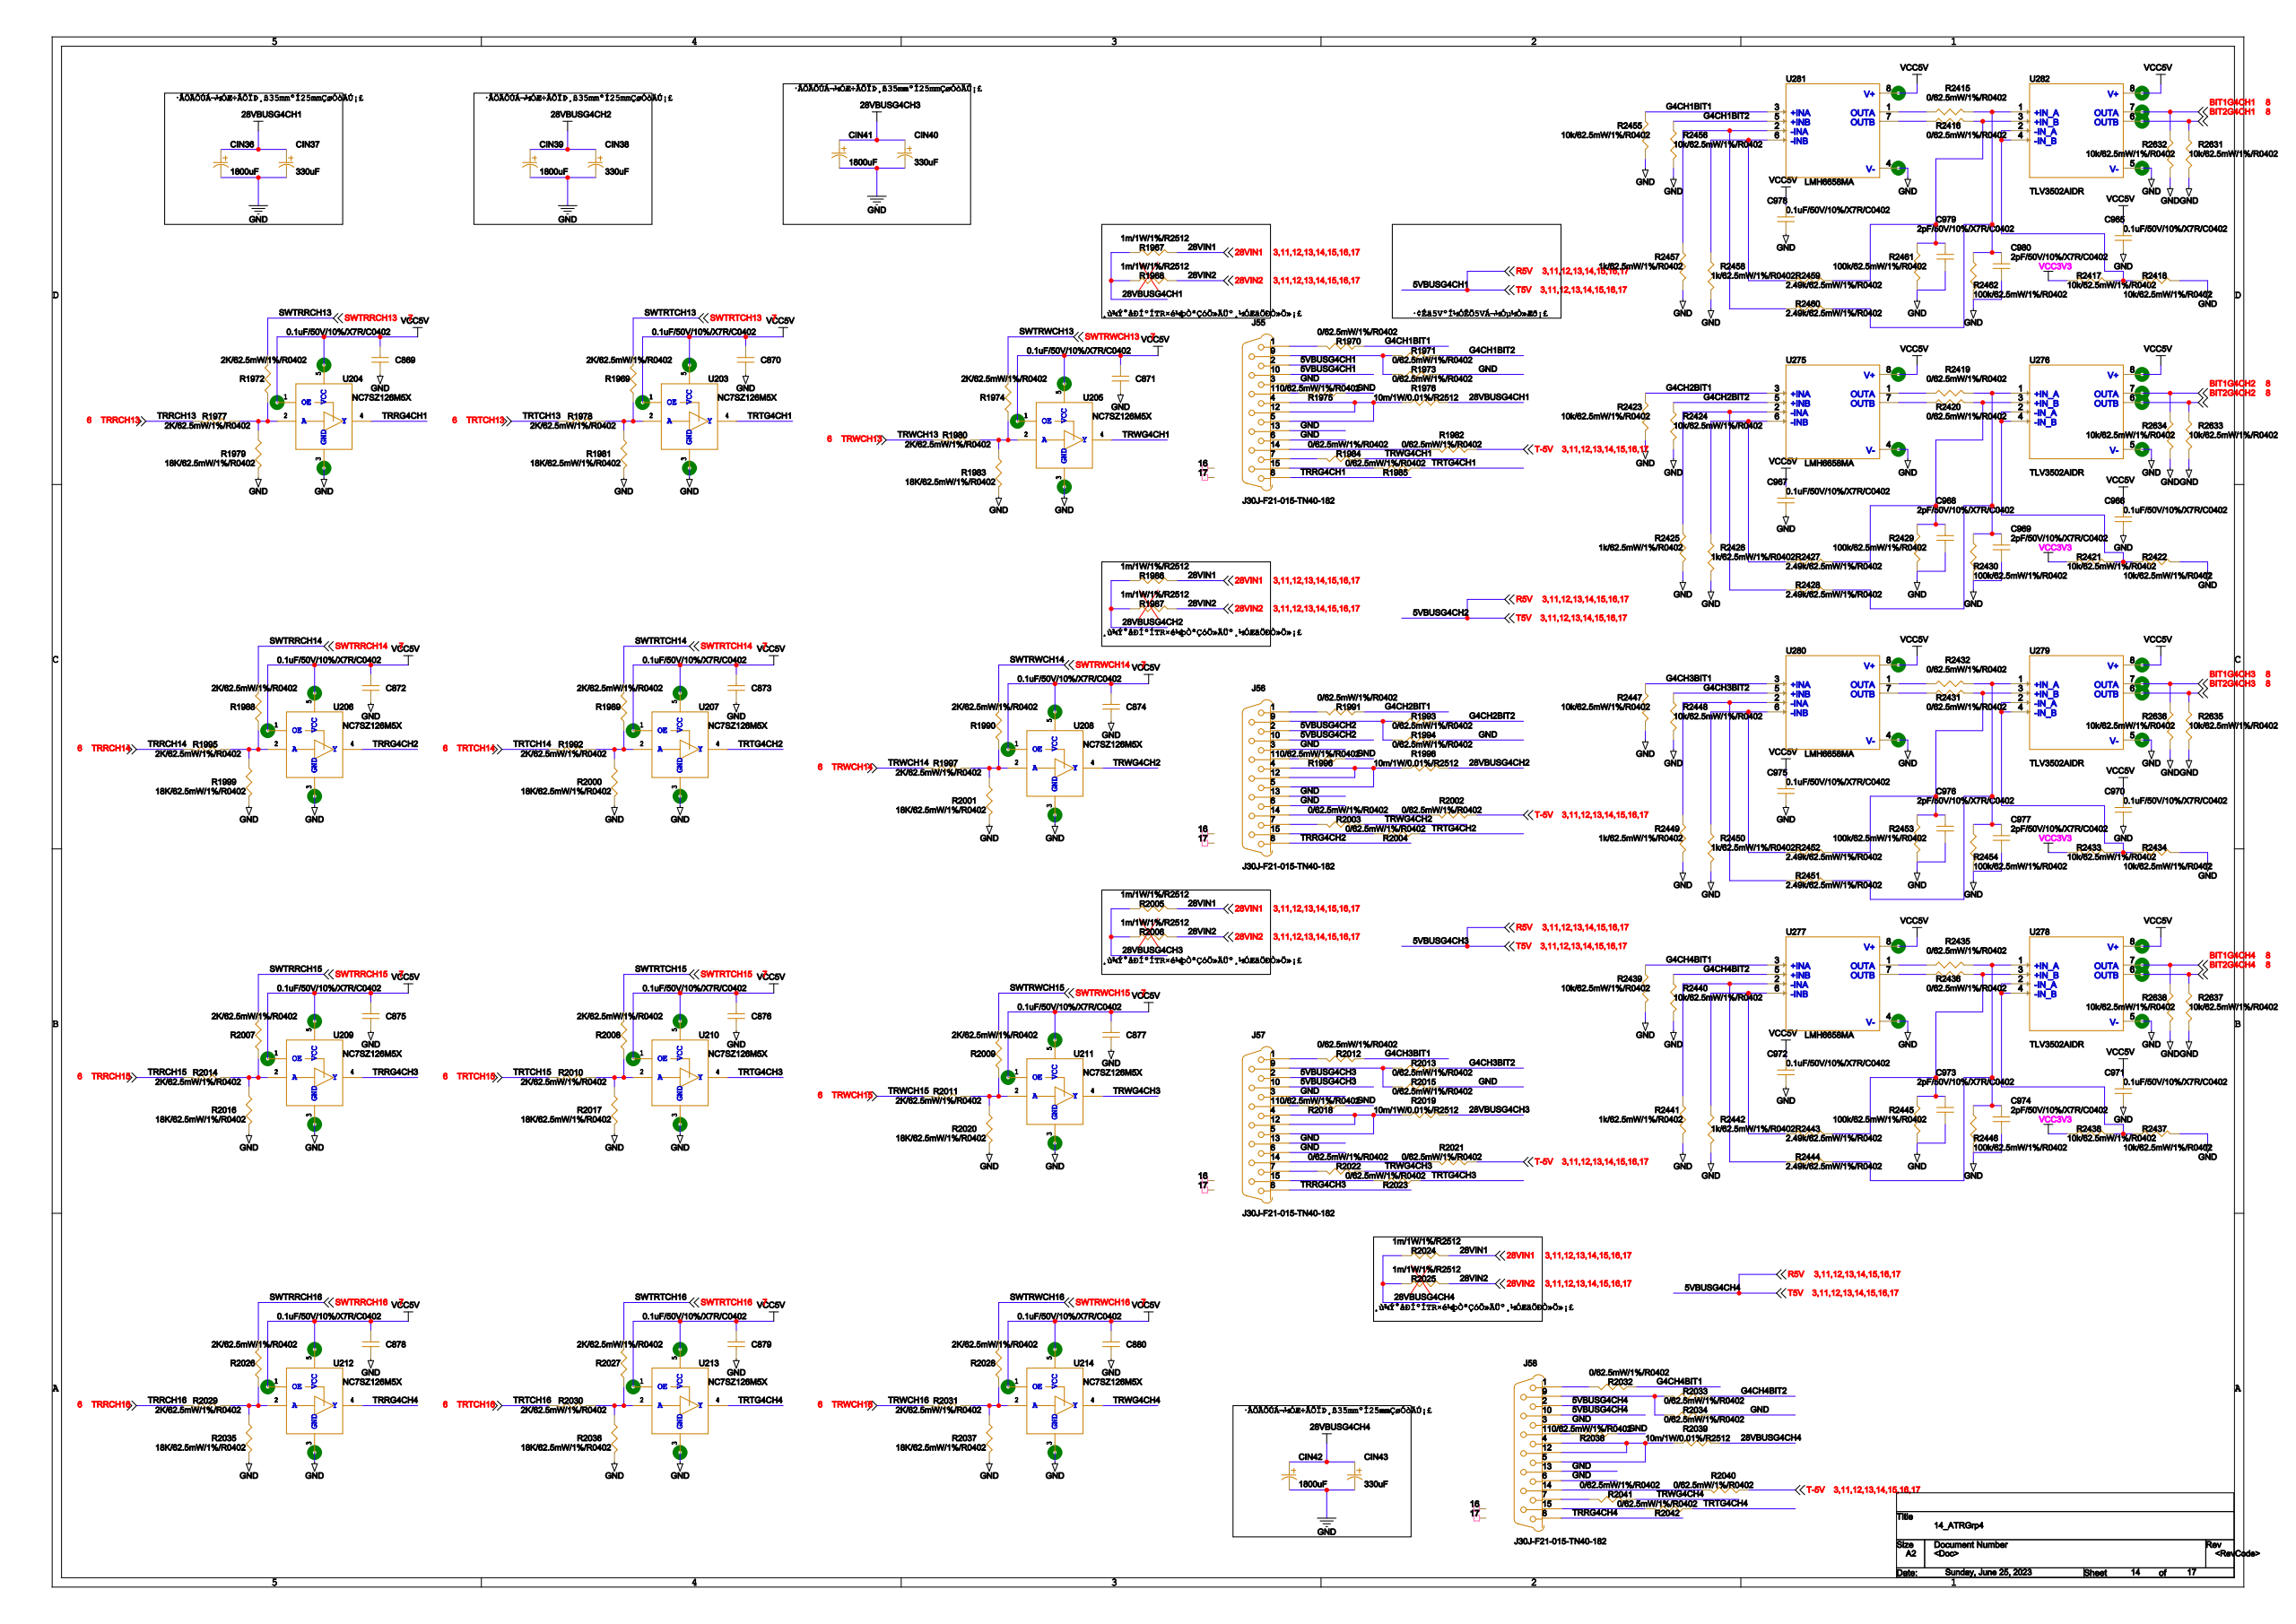Circuit board | Cadence Allegro | 2002 parts | 1538 nets | one sheet of the schematic
Parts on this sheet (reference | value | footprint):
C869 | 0.1uF/50V/10%/X7R/C0402 | 0402
C870 | 0.1uF/50V/10%/X7R/C0402 | 0402
C871 | 0.1uF/50V/10%/X7R/C0402 | 0402
C872 | 0.1uF/50V/10%/X7R/C0402 | 0402
C873 | 0.1uF/50V/10%/X7R/C0402 | 0402
C874 | 0.1uF/50V/10%/X7R/C0402 | 0402
C875 | 0.1uF/50V/10%/X7R/C0402 | 0402
C876 | 0.1uF/50V/10%/X7R/C0402 | 0402
C877 | 0.1uF/50V/10%/X7R/C0402 | 0402
C878 | 0.1uF/50V/10%/X7R/C0402 | 0402
C879 | 0.1uF/50V/10%/X7R/C0402 | 0402
C880 | 0.1uF/50V/10%/X7R/C0402 | 0402
C965 | 0.1uF/50V/10%/X7R/C0402 | 0402
C966 | 0.1uF/50V/10%/X7R/C0402 | 0402
C968 | 2pF/50V/10%/X7R/C0402 | 0402
C969 | 2pF/50V/10%/X7R/C0402 | 0402
C970 | 0.1uF/50V/10%/X7R/C0402 | 0402
C971 | 0.1uF/50V/10%/X7R/C0402 | 0402
C973 | 2pF/50V/10%/X7R/C0402 | 0402
C974 | 2pF/50V/10%/X7R/C0402 | 0402
C976 | 2pF/50V/10%/X7R/C0402 | 0402
C977 | 2pF/50V/10%/X7R/C0402 | 0402
C979 | 2pF/50V/10%/X7R/C0402 | 0402
C980 | 2pF/50V/10%/X7R/C0402 | 0402
CIN36 | ECF1HM182M27OTPO | AP-SMD_BD18-L27-W6_6-LS7_21
CIN37 | ECF1JM331G20OTPO | AP-SMD_BD10-L20-W6_6-LS7_21
CIN38 | ECF1JM331G20OTPO | AP-SMD_BD10-L20-W6_6-LS7_21
CIN39 | ECF1HM182M27OTPO | AP-SMD_BD18-L27-W6_6-LS7_21
CIN40 | ECF1JM331G20OTPO | AP-SMD_BD10-L20-W6_6-LS7_21
CIN41 | ECF1HM182M27OTPO | AP-SMD_BD18-L27-W6_6-LS7_21
CIN42 | ECF1HM182M27OTPO | AP-SMD_BD18-L27-W6_6-LS7_21
CIN43 | ECF1JM331G20OTPO | AP-SMD_BD10-L20-W6_6-LS7_21
J55 | J30J-F21-015-TN40-182 | J30J-F21-015-TN40-182
J56 | J30J-F21-015-TN40-182 | J30J-F21-015-TN40-182
J57 | J30J-F21-015-TN40-182 | J30J-F21-015-TN40-182
J58 | J30J-F21-015-TN40-182 | J30J-F21-015-TN40-182
R1967 | 1m/1W/1%/R2512 | 2512
R1968 | 1m/1W/1%/R2512 | 2512
R1969 | 2K/62.5mW/1%/R0402 | 0402
R1970 | 0/62.5mW/1%/R0402 | 0402
R1971 | 0/62.5mW/1%/R0402 | 0402
R1972 | 2K/62.5mW/1%/R0402 | 0402
R1973 | 0/62.5mW/1%/R0402 | 0402
R1974 | 2K/62.5mW/1%/R0402 | 0402
R1975 | 0/62.5mW/1%/R0402 | 0402
R1976 | 10m/1W/0.01%/R2512 | 2512
R1977 | 2K/62.5mW/1%/R0402 | 0402
R1978 | 2K/62.5mW/1%/R0402 | 0402
R1979 | 18K/62.5mW/1%/R0402 | 0402
R1980 | 2K/62.5mW/1%/R0402 | 0402
R1981 | 18K/62.5mW/1%/R0402 | 0402
R1982 | 0/62.5mW/1%/R0402 | 0402
R1983 | 18K/62.5mW/1%/R0402 | 0402
R1984 | 0/62.5mW/1%/R0402 | 0402
R1985 | 0/62.5mW/1%/R0402 | 0402
R1986 | 1m/1W/1%/R2512 | 2512
R1987 | 1m/1W/1%/R2512 | 2512
R1988 | 2K/62.5mW/1%/R0402 | 0402
R1989 | 2K/62.5mW/1%/R0402 | 0402
R1990 | 2K/62.5mW/1%/R0402 | 0402
R1991 | 0/62.5mW/1%/R0402 | 0402
R1992 | 2K/62.5mW/1%/R0402 | 0402
R1993 | 0/62.5mW/1%/R0402 | 0402
R1994 | 0/62.5mW/1%/R0402 | 0402
R1995 | 2K/62.5mW/1%/R0402 | 0402
R1996 | 0/62.5mW/1%/R0402 | 0402
R1997 | 2K/62.5mW/1%/R0402 | 0402
R1998 | 10m/1W/0.01%/R2512 | 2512
R1999 | 18K/62.5mW/1%/R0402 | 0402
R2000 | 18K/62.5mW/1%/R0402 | 0402
R2001 | 18K/62.5mW/1%/R0402 | 0402
R2002 | 0/62.5mW/1%/R0402 | 0402
R2003 | 0/62.5mW/1%/R0402 | 0402
R2004 | 0/62.5mW/1%/R0402 | 0402
R2005 | 1m/1W/1%/R2512 | 2512
R2006 | 1m/1W/1%/R2512 | 2512
R2007 | 2K/62.5mW/1%/R0402 | 0402
R2008 | 2K/62.5mW/1%/R0402 | 0402
R2009 | 2K/62.5mW/1%/R0402 | 0402
R2010 | 2K/62.5mW/1%/R0402 | 0402
R2011 | 2K/62.5mW/1%/R0402 | 0402
R2012 | 0/62.5mW/1%/R0402 | 0402
R2013 | 0/62.5mW/1%/R0402 | 0402
R2014 | 2K/62.5mW/1%/R0402 | 0402
R2015 | 0/62.5mW/1%/R0402 | 0402
R2016 | 18K/62.5mW/1%/R0402 | 0402
R2017 | 18K/62.5mW/1%/R0402 | 0402
R2018 | 0/62.5mW/1%/R0402 | 0402
R2019 | 10m/1W/0.01%/R2512 | 2512
R2020 | 18K/62.5mW/1%/R0402 | 0402
R2021 | 0/62.5mW/1%/R0402 | 0402
R2022 | 0/62.5mW/1%/R0402 | 0402
R2023 | 0/62.5mW/1%/R0402 | 0402
R2024 | 1m/1W/1%/R2512 | 2512
R2025 | 1m/1W/1%/R2512 | 2512
R2026 | 2K/62.5mW/1%/R0402 | 0402
R2027 | 2K/62.5mW/1%/R0402 | 0402
R2028 | 2K/62.5mW/1%/R0402 | 0402
R2029 | 2K/62.5mW/1%/R0402 | 0402
R2030 | 2K/62.5mW/1%/R0402 | 0402
R2031 | 2K/62.5mW/1%/R0402 | 0402
R2032 | 0/62.5mW/1%/R0402 | 0402
R2033 | 0/62.5mW/1%/R0402 | 0402
R2034 | 0/62.5mW/1%/R0402 | 0402
R2035 | 18K/62.5mW/1%/R0402 | 0402
R2036 | 18K/62.5mW/1%/R0402 | 0402
R2037 | 18K/62.5mW/1%/R0402 | 0402
R2038 | 0/62.5mW/1%/R0402 | 0402
R2039 | 10m/1W/0.01%/R2512 | 2512
R2040 | 0/62.5mW/1%/R0402 | 0402
R2041 | 0/62.5mW/1%/R0402 | 0402
R2042 | 0/62.5mW/1%/R0402 | 0402
R2415 | 0/62.5mW/1%/R0402 | 0402
R2416 | 0/62.5mW/1%/R0402 | 0402
R2417 | 10k/62.5mW/1%/R0402 | 0402
R2418 | 10k/62.5mW/1%/R0402 | 0402
R2419 | 0/62.5mW/1%/R0402 | 0402
R2420 | 0/62.5mW/1%/R0402 | 0402
R2421 | 10k/62.5mW/1%/R0402 | 0402
R2422 | 10k/62.5mW/1%/R0402 | 0402
R2423 | 10k/62.5mW/1%/R0402 | 0402
R2424 | 10k/62.5mW/1%/R0402 | 0402
R2425 | 1K/62.5mW/1%/R0402 | 0402
R2426 | 1K/62.5mW/1%/R0402 | 0402
R2428 | 2.49k/62.5mW/1%/R0402 | 0402
R2429 | 100k/62.5mW/1%/R0402 | 0402
R2430 | 100k/62.5mW/1%/R0402 | 0402
R2431 | 0/62.5mW/1%/R0402 | 0402
R2432 | 0/62.5mW/1%/R0402 | 0402
R2433 | 10k/62.5mW/1%/R0402 | 0402
R2434 | 10k/62.5mW/1%/R0402 | 0402
R2435 | 0/62.5mW/1%/R0402 | 0402
R2436 | 0/62.5mW/1%/R0402 | 0402
R2437 | 10k/62.5mW/1%/R0402 | 0402
R2438 | 10k/62.5mW/1%/R0402 | 0402
R2439 | 10k/62.5mW/1%/R0402 | 0402
R2440 | 10k/62.5mW/1%/R0402 | 0402
R2441 | 1K/62.5mW/1%/R0402 | 0402
R2442 | 1K/62.5mW/1%/R0402 | 0402
R2444 | 2.49k/62.5mW/1%/R0402 | 0402
R2445 | 100k/62.5mW/1%/R0402 | 0402
R2446 | 100k/62.5mW/1%/R0402 | 0402
R2447 | 10k/62.5mW/1%/R0402 | 0402
R2448 | 10k/62.5mW/1%/R0402 | 0402
R2449 | 1K/62.5mW/1%/R0402 | 0402
R2450 | 1K/62.5mW/1%/R0402 | 0402
R2451 | 2.49k/62.5mW/1%/R0402 | 0402
R2452 | 2.49k/62.5mW/1%/R0402 | 0402
R2453 | 100k/62.5mW/1%/R0402 | 0402
R2454 | 100k/62.5mW/1%/R0402 | 0402
R2455 | 10k/62.5mW/1%/R0402 | 0402
R2456 | 10k/62.5mW/1%/R0402 | 0402
R2457 | 1K/62.5mW/1%/R0402 | 0402
R2458 | 1K/62.5mW/1%/R0402 | 0402
R2460 | 2.49k/62.5mW/1%/R0402 | 0402
R2461 | 100k/62.5mW/1%/R0402 | 0402
R2462 | 100k/62.5mW/1%/R0402 | 0402
R2631 | 10k/62.5mW/1%/R0402 | 0402
R2632 | 10k/62.5mW/1%/R0402 | 0402
R2633 | 10k/62.5mW/1%/R0402 | 0402
R2634 | 10k/62.5mW/1%/R0402 | 0402
R2635 | 10k/62.5mW/1%/R0402 | 0402
R2636 | 10k/62.5mW/1%/R0402 | 0402
R2637 | 10k/62.5mW/1%/R0402 | 0402
R2638 | 10k/62.5mW/1%/R0402 | 0402
U203 | NC7SZ126M5X | SOT-23-5
U204 | NC7SZ126M5X | SOT-23-5
U205 | NC7SZ126M5X | SOT-23-5
U206 | NC7SZ126M5X | SOT-23-5
U207 | NC7SZ126M5X | SOT-23-5
U208 | NC7SZ126M5X | SOT-23-5
U209 | NC7SZ126M5X | SOT-23-5
U210 | NC7SZ126M5X | SOT-23-5
U211 | NC7SZ126M5X | SOT-23-5
U212 | NC7SZ126M5X | SOT-23-5
U213 | NC7SZ126M5X | SOT-23-5
U214 | NC7SZ126M5X | SOT-23-5
U275 | LMH6658MA | SOIC127P599X175-8N
U277 | LMH6658MA | SOIC127P599X175-8N
U279 | TLV3502AIDR | SOIC127P599X175-8N
U281 | LMH6658MA | SOIC127P599X175-8N
Nets of these parts (net: part-pin ...):
3.3V: R2417-1 R2421-1 R2433-1 R2438-1
AGND: C869-2 C870-2 C871-2 C872-2 C873-2 C874-2 C875-2 C876-2 C877-2 C878-2 C879-2 C880-2 C965-2 C966-2 C968-2 C969-2 C970-2 C971-2 C973-2 C974-2 C976-2 C977-2 C979-2 C980-2 CIN36-2 CIN37-2 CIN38-2 CIN39-2 CIN40-2 CIN41-2 CIN42-2 CIN43-2 J55-3 J55-6 J55-13 J56-3 J56-6 J56-13 J57-3 J57-6 J57-13 J58-3 J58-6 J58-13 R1973-1 R1975-1 R1979-1 R1981-1 R1983-1 R1994-1 R1996-1 R1999-1 R2000-1 R2001-1 R2015-1 R2016-1 R2017-1 R2018-1 R2020-1 R2034-1 R2035-1 R2036-1 R2037-1 R2038-1 R2418-2 R2422-2 R2423-2 R2424-2 R2425-2 R2426-2 R2429-2 R2430-2 R2434-2 R2437-2 R2439-2 R2440-2 R2441-2 R2442-2 R2445-2 R2446-2 R2447-2 R2448-2 R2449-2 R2450-2 R2453-2 R2454-2 R2455-2 R2456-2 R2457-2 R2458-2 R2461-2 R2462-2 R2631-2 R2632-2 R2633-2 R2634-2 R2635-2 R2636-2 R2637-2 R2638-2 U203-3 U204-3 U205-3 U206-3 U207-3 U208-3 U209-3 U210-3 U211-3 U212-3 U213-3 U214-3 U275-4 U277-4 U279-5 U281-4
VCC5V: C869-1 C870-1 C871-1 C872-1 C873-1 C874-1 C875-1 C876-1 C877-1 C878-1 C879-1 C880-1 C965-1 C966-1 C970-1 C971-1 U203-1 U203-5 U204-1 U204-5 U205-1 U205-5 U206-1 U206-5 U207-1 U207-5 U208-1 U208-5 U209-1 U209-5 U210-1 U210-5 U211-1 U211-5 U212-1 U212-5 U213-1 U213-5 U214-1 U214-5 U275-8 U277-8 U279-8 U281-8
28VIN1: R1967-2 R1968-2 R1986-2 R1987-2 R2005-2 R2006-2 R2024-2 R2025-2
R5V: J55-2 J55-10 J56-2 J56-10 J57-2 J57-10 J58-2 J58-10
T-5V: R1982-1 R2002-1 R2021-1 R2040-1
N24402779: R2426-1 U275-6
N24402789: C968-1 R2420-2 R2429-1
N24402767: R2425-1 R2428-1 U275-2
N24402787: C969-1 R2419-2 R2428-2 R2430-1
N24403333: R2442-1 U277-6
N24403343: C973-1 R2436-2 R2445-1
N24403321: R2441-1 R2444-1 U277-2
N24403341: C974-1 R2435-2 R2444-2 R2446-1
N24403145: R2449-1 R2451-1
N24403161: C977-1 R2432-2 R2451-2 R2454-1 U279-1
N24403149: R2450-1 R2452-1
N24403163: C976-1 R2431-2 R2452-2 R2453-1 U279-3
N24402599: R2458-1 U281-6
N24402609: C979-1 R2416-2 R2461-1
N24402595: R2457-1 R2460-1 U281-2
N24402607: C980-1 R2415-2 R2460-2 R2462-1
G4CH2BIT1: R1991-1 R2423-1 U275-3
G4CH2BIT2: R1993-1 R2424-1 U275-5
N24402783: R2419-1 U275-1
N24402785: R2420-1 U275-7
G4CH4BIT1: R2032-1 R2439-1 U277-3
G4CH4BIT2: R2033-1 R2440-1 U277-5
N24403337: R2435-1 U277-1
N24403339: R2436-1 U277-7
G4CH3BIT1: R2012-1 R2447-1
G4CH3BIT2: R2013-1 R2448-1
N24403157: R2432-1
N24403159: R2431-1
G4CH1BIT1: R1970-1 R2455-1 U281-3
G4CH1BIT2: R1971-1 R2456-1 U281-5
N24402603: R2415-1 U281-1
N24402605: R2416-1 U281-7
N24402841: R2421-2 R2422-1
BIT1G4CH2: R2634-1
BIT2G4CH2: R2633-1
N24403395: R2437-1 R2438-2
BIT1G4CH4: R2638-1
BIT2G4CH4: R2637-1
N24403215: R2433-2 R2434-1 U279-2 U279-4
BIT1G4CH3: R2636-1 U279-7
BIT2G4CH3: R2635-1 U279-6
N24402661: R2417-2 R2418-1
BIT1G4CH1: R2632-1
BIT2G4CH1: R2631-1
N23728226: J55-1 R1970-2
N23728239: J55-11 R1975-2
N23728241: J55-4 J55-5 J55-12 R1976-1
N23728253: J55-14 R1982-2
N23728257: J55-15 R1985-2
N23728255: J55-7 R1984-2
TRRG4CH1: J55-8 U204-4
N23728228: J55-9 R1971-2 R1973-2
N23728785: J56-1 R1991-2
N23728798: J56-11 R1996-2
N23728800: J56-4 J56-5 J56-12 R1998-1
N23728812: J56-14 R2002-2
N23728816: J56-15 R2004-2
N23728814: J56-7 R2003-2
TRRG4CH2: J56-8 U206-4
N23728787: J56-9 R1993-2 R1994-2
N23729412: J57-1 R2012-2
N23729425: J57-11 R2018-2
N23729427: J57-4 J57-5 J57-12 R2019-1
N23729439: J57-14 R2021-2
N23729443: J57-15 R2023-2
N23729441: J57-7 R2022-2
TRRG4CH3: J57-8 U209-4
N23729414: J57-9 R2013-2 R2015-2
N23730216: J58-1 R2032-2
N23730229: J58-11 R2038-2
N23730231: J58-4 J58-5 J58-12 R2039-1
N23730243: J58-14 R2040-2
N23730247: J58-15 R2042-2
N23730245: J58-7 R2041-2
TRRG4CH4: J58-8 U212-4
N23730218: J58-9 R2033-2 R2034-2
28VBUSG4CH1: CIN36-1 CIN37-1 R1967-1 R1968-1 R1976-2
28VBUSG4CH2: CIN38-1 CIN39-1 R1986-1 R1987-1 R1998-2
28VBUSG4CH3: CIN40-1 CIN41-1 R2005-1 R2006-1 R2019-2
28VBUSG4CH4: CIN42-1 CIN43-1 R2024-1 R2025-1 R2039-2
SWTRTCH13: R1969-1
N24010050: R1969-2 R1978-2 R1981-2 U203-2
SWTRRCH13: R1972-1
N24011030: R1972-2 R1977-2 R1979-2 U204-2
SWTRWCH13: R1974-1
N24010538: R1974-2 R1980-2 R1983-2 U205-2
TRRCH13: R1977-1
TRTCH13: R1978-1
TRWCH13: R1980-1
SWTRRCH14: R1988-1
N24011148: R1988-2 R1995-2 R1999-2 U206-2
SWTRTCH14: R1989-1
N24010168: R1989-2 R1992-2 R2000-2 U207-2
SWTRWCH14: R1990-1
N24010660: R1990-2 R1997-2 R2001-2 U208-2
TRTCH14: R1992-1
TRRCH14: R1995-1
TRWCH14: R1997-1
SWTRRCH15: R2007-1
N24011274: R2007-2 R2014-2 R2016-2 U209-2
SWTRTCH15: R2008-1
N24010294: R2008-2 R2010-2 R2017-2 U210-2
SWTRWCH15: R2009-1
N24010782: R2009-2 R2011-2 R2020-2 U211-2
TRTCH15: R2010-1
TRWCH15: R2011-1
TRRCH15: R2014-1
SWTRRCH16: R2026-1
N24011392: R2026-2 R2029-2 R2035-2 U212-2
SWTRTCH16: R2027-1
N24010416: R2027-2 R2030-2 R2036-2 U213-2
SWTRWCH16: R2028-1
N24010904: R2028-2 R2031-2 R2037-2 U214-2
TRRCH16: R2029-1
TRTCH16: R2030-1
TRWCH16: R2031-1
TRTG4CH1: R1985-1 U203-4
TRWG4CH1: R1984-1 U205-4
TRTG4CH2: R2004-1 U207-4
TRWG4CH2: R2003-1 U208-4
TRTG4CH3: R2023-1 U210-4
TRWG4CH3: R2022-1 U211-4
TRTG4CH4: R2042-1 U213-4
TRWG4CH4: R2041-1 U214-4